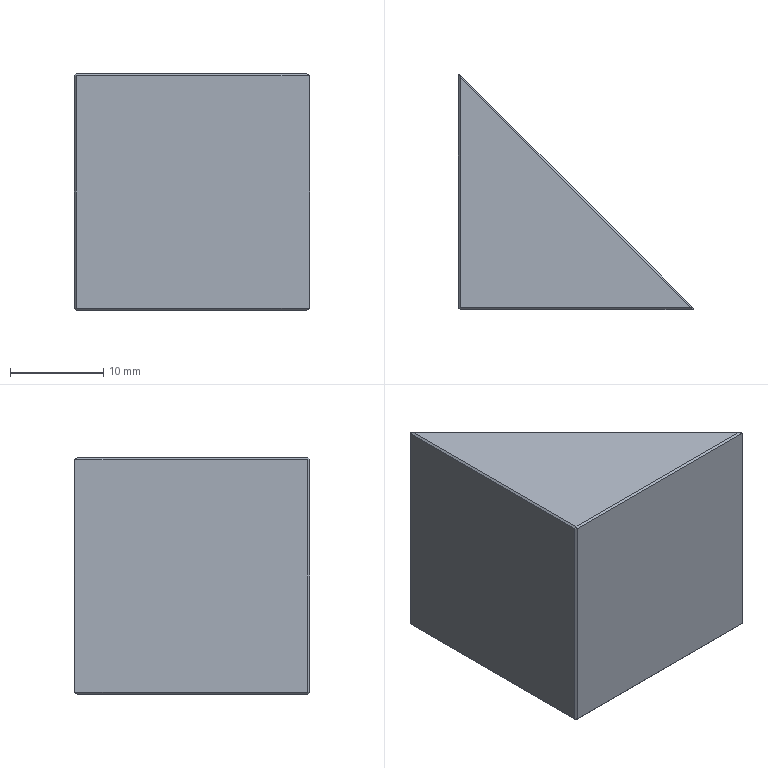Part | STEP file | PBS24-532-HP-1-0.step.STEP.STEP-259.STEP | 1 solid | 20 faces | box 25.259 x 25.259 x 25.4 mm | volume 8189 mm3 | plane 20
STEP:
#1=CARTESIAN_POINT('',(25.201,0.002851,25.203));
#2=VERTEX_POINT('',#1);
#3=CARTESIAN_POINT('',(25.257,0.1386,25.203));
#4=VERTEX_POINT('',#3);
#5=CARTESIAN_POINT('',(25.259,0.1414,25.203));
#6=DIRECTION('',(0.3827,0.9239,0.));
#7=VECTOR('',#6,1000.);
#8=LINE('',#5,#7);
#9=EDGE_CURVE('',#2,#4,#8,.T.);
#10=ORIENTED_EDGE('',*,*,#9,.F.);
#11=CARTESIAN_POINT('',(25.2,0.,25.2));
#12=VERTEX_POINT('',#11);
#13=CARTESIAN_POINT('',(25.27,0.1684,25.368));
#14=DIRECTION('',(-0.2811,-0.6786,-0.6786));
#15=VECTOR('',#14,1000.);
#16=LINE('',#13,#15);
#17=EDGE_CURVE('',#2,#12,#16,.T.);
#18=ORIENTED_EDGE('',*,*,#17,.T.);
#19=CARTESIAN_POINT('',(25.2,0.,0.2));
#20=VERTEX_POINT('',#19);
#21=CARTESIAN_POINT('',(25.2,0.,25.4));
#22=DIRECTION('',(0.,0.,1.));
#23=VECTOR('',#22,1000.);
#24=LINE('',#21,#23);
#25=EDGE_CURVE('',#20,#12,#24,.T.);
#26=ORIENTED_EDGE('',*,*,#25,.F.);
#27=CARTESIAN_POINT('',(25.201,0.002851,0.1971));
#28=VERTEX_POINT('',#27);
#29=CARTESIAN_POINT('',(20.425,-11.528,11.728));
#30=DIRECTION('',(0.2811,0.6786,-0.6786));
#31=VECTOR('',#30,1000.);
#32=LINE('',#29,#31);
#33=EDGE_CURVE('',#20,#28,#32,.T.);
#34=ORIENTED_EDGE('',*,*,#33,.T.);
#35=CARTESIAN_POINT('',(25.257,0.1386,0.1971));
#36=VERTEX_POINT('',#35);
#37=CARTESIAN_POINT('',(25.259,0.1414,0.1971));
#38=DIRECTION('',(0.3827,0.9239,0.));
#39=VECTOR('',#38,1000.);
#40=LINE('',#37,#39);
#41=EDGE_CURVE('',#28,#36,#40,.T.);
#42=ORIENTED_EDGE('',*,*,#41,.T.);
#43=CARTESIAN_POINT('',(25.259,0.1414,0.2));
#44=VERTEX_POINT('',#43);
#45=CARTESIAN_POINT('',(28.081,6.955,7.014));
#46=DIRECTION('',(-0.2811,-0.6786,-0.6786));
#47=VECTOR('',#46,1000.);
#48=LINE('',#45,#47);
#49=EDGE_CURVE('',#44,#36,#48,.T.);
#50=ORIENTED_EDGE('',*,*,#49,.F.);
#51=CARTESIAN_POINT('',(25.259,0.1414,25.2));
#52=VERTEX_POINT('',#51);
#53=CARTESIAN_POINT('',(25.259,0.1414,25.4));
#54=DIRECTION('',(0.,0.,-1.));
#55=VECTOR('',#54,1000.);
#56=LINE('',#53,#55);
#57=EDGE_CURVE('',#52,#44,#56,.T.);
#58=ORIENTED_EDGE('',*,*,#57,.F.);
#59=CARTESIAN_POINT('',(26.586,3.345,21.996));
#60=DIRECTION('',(0.2811,0.6786,-0.6786));
#61=VECTOR('',#60,1000.);
#62=LINE('',#59,#61);
#63=EDGE_CURVE('',#4,#52,#62,.T.);
#64=ORIENTED_EDGE('',*,*,#63,.F.);
#65=EDGE_LOOP('',(#10,#18,#26,#34,#42,#50,#58,#64));
#66=FACE_OUTER_BOUND('',#65,.T.);
#67=CARTESIAN_POINT('',(25.259,0.1414,25.4));
#68=DIRECTION('',(-0.9239,0.3827,0.));
#69=DIRECTION('',(0.,0.,1.));
#70=AXIS2_PLACEMENT_3D('',#67,#68,#69);
#71=PLANE('',#70);
#72=ADVANCED_FACE('',(#66),#71,.F.);
#73=CARTESIAN_POINT('',(24.919,0.1994,0.0006229));
#74=VERTEX_POINT('',#73);
#75=CARTESIAN_POINT('',(24.917,0.2,0.));
#76=VERTEX_POINT('',#75);
#77=CARTESIAN_POINT('',(-1.344,11.078,-10.878));
#78=DIRECTION('',(-0.8629,0.3574,-0.3574));
#79=VECTOR('',#78,1000.);
#80=LINE('',#77,#79);
#81=EDGE_CURVE('',#74,#76,#80,.T.);
#82=ORIENTED_EDGE('',*,*,#81,.F.);
#83=CARTESIAN_POINT('',(12.396,8.91,-8.71));
#84=DIRECTION('',(0.7129,-0.4959,0.4959));
#85=VECTOR('',#84,1000.);
#86=LINE('',#83,#85);
#87=EDGE_CURVE('',#74,#28,#86,.T.);
#88=ORIENTED_EDGE('',*,*,#87,.T.);
#89=ORIENTED_EDGE('',*,*,#33,.F.);
#90=CARTESIAN_POINT('',(0.2,0.,0.2));
#91=VERTEX_POINT('',#90);
#92=CARTESIAN_POINT('',(25.117,0.,0.2));
#93=DIRECTION('',(1.,0.,0.));
#94=VECTOR('',#93,1000.);
#95=LINE('',#92,#94);
#96=EDGE_CURVE('',#91,#20,#95,.T.);
#97=ORIENTED_EDGE('',*,*,#96,.F.);
#98=CARTESIAN_POINT('',(0.1981,0.00185,0.1981));
#99=VERTEX_POINT('',#98);
#100=CARTESIAN_POINT('',(8.6,-8.4,8.6));
#101=DIRECTION('',(0.5774,-0.5774,0.5774));
#102=VECTOR('',#101,1000.);
#103=LINE('',#100,#102);
#104=EDGE_CURVE('',#99,#91,#103,.T.);
#105=ORIENTED_EDGE('',*,*,#104,.F.);
#106=CARTESIAN_POINT('',(0.1981,0.1981,0.00185));
#107=VERTEX_POINT('',#106);
#108=CARTESIAN_POINT('',(0.1981,0.,0.2));
#109=DIRECTION('',(0.,0.7071,-0.7071));
#110=VECTOR('',#109,1000.);
#111=LINE('',#108,#110);
#112=EDGE_CURVE('',#99,#107,#111,.T.);
#113=ORIENTED_EDGE('',*,*,#112,.T.);
#114=CARTESIAN_POINT('',(0.2,0.2,0.));
#115=VERTEX_POINT('',#114);
#116=CARTESIAN_POINT('',(0.,0.,0.2));
#117=DIRECTION('',(-0.5774,-0.5774,0.5774));
#118=VECTOR('',#117,1000.);
#119=LINE('',#116,#118);
#120=EDGE_CURVE('',#115,#107,#119,.T.);
#121=ORIENTED_EDGE('',*,*,#120,.F.);
#122=CARTESIAN_POINT('',(0.2,0.2,0.));
#123=DIRECTION('',(-1.,0.,0.));
#124=VECTOR('',#123,1000.);
#125=LINE('',#122,#124);
#126=EDGE_CURVE('',#76,#115,#125,.T.);
#127=ORIENTED_EDGE('',*,*,#126,.F.);
#128=EDGE_LOOP('',(#82,#88,#89,#97,#105,#113,#121,#127));
#129=FACE_OUTER_BOUND('',#128,.T.);
#130=CARTESIAN_POINT('',(0.,0.,0.2));
#131=DIRECTION('',(0.,-0.7071,-0.7071));
#132=DIRECTION('',(0.,-0.7071,0.7071));
#133=AXIS2_PLACEMENT_3D('',#130,#131,#132);
#134=PLANE('',#133);
#135=ADVANCED_FACE('',(#129),#134,.T.);
#136=ORIENTED_EDGE('',*,*,#49,.T.);
#137=CARTESIAN_POINT('',(3.494,4.045,-12.429));
#138=DIRECTION('',(-0.8547,0.1534,-0.4959));
#139=VECTOR('',#138,1000.);
#140=LINE('',#137,#139);
#141=EDGE_CURVE('',#36,#74,#140,.T.);
#142=ORIENTED_EDGE('',*,*,#141,.T.);
#143=ORIENTED_EDGE('',*,*,#81,.T.);
#144=CARTESIAN_POINT('',(0.2,24.917,0.));
#145=VERTEX_POINT('',#144);
#146=CARTESIAN_POINT('',(25.259,-0.1414,0.));
#147=DIRECTION('',(0.7071,-0.7071,0.));
#148=VECTOR('',#147,1000.);
#149=LINE('',#146,#148);
#150=EDGE_CURVE('',#145,#76,#149,.T.);
#151=ORIENTED_EDGE('',*,*,#150,.F.);
#152=CARTESIAN_POINT('',(0.1994,24.919,0.0006229));
#153=VERTEX_POINT('',#152);
#154=CARTESIAN_POINT('',(0.,25.4,0.2));
#155=DIRECTION('',(-0.3574,0.8629,0.3574));
#156=VECTOR('',#155,1000.);
#157=LINE('',#154,#156);
#158=EDGE_CURVE('',#145,#153,#157,.T.);
#159=ORIENTED_EDGE('',*,*,#158,.T.);
#160=CARTESIAN_POINT('',(0.1386,25.257,0.1971));
#161=VERTEX_POINT('',#160);
#162=CARTESIAN_POINT('',(0.1164,25.381,0.2688));
#163=DIRECTION('',(-0.1534,0.8547,0.4959));
#164=VECTOR('',#163,1000.);
#165=LINE('',#162,#164);
#166=EDGE_CURVE('',#153,#161,#165,.T.);
#167=ORIENTED_EDGE('',*,*,#166,.T.);
#168=CARTESIAN_POINT('',(0.1414,25.259,0.2));
#169=VERTEX_POINT('',#168);
#170=CARTESIAN_POINT('',(0.1033,25.243,0.1619));
#171=DIRECTION('',(0.6786,0.2811,0.6786));
#172=VECTOR('',#171,1000.);
#173=LINE('',#170,#172);
#174=EDGE_CURVE('',#161,#169,#173,.T.);
#175=ORIENTED_EDGE('',*,*,#174,.T.);
#176=CARTESIAN_POINT('',(0.,25.4,0.2));
#177=DIRECTION('',(-0.7071,0.7071,0.));
#178=VECTOR('',#177,1000.);
#179=LINE('',#176,#178);
#180=EDGE_CURVE('',#44,#169,#179,.T.);
#181=ORIENTED_EDGE('',*,*,#180,.F.);
#182=EDGE_LOOP('',(#136,#142,#143,#151,#159,#167,#175,#181));
#183=FACE_OUTER_BOUND('',#182,.T.);
#184=CARTESIAN_POINT('',(0.,25.4,0.2));
#185=DIRECTION('',(0.5,0.5,-0.7071));
#186=DIRECTION('',(-0.8165,0.,-0.5774));
#187=AXIS2_PLACEMENT_3D('',#184,#185,#186);
#188=PLANE('',#187);
#189=ADVANCED_FACE('',(#183),#188,.T.);
#190=CARTESIAN_POINT('',(0.,25.2,0.2));
#191=VERTEX_POINT('',#190);
#192=CARTESIAN_POINT('',(0.002851,25.201,0.1971));
#193=VERTEX_POINT('',#192);
#194=CARTESIAN_POINT('',(-4.807,23.209,5.007));
#195=DIRECTION('',(0.6786,0.2811,-0.6786));
#196=VECTOR('',#195,1000.);
#197=LINE('',#194,#196);
#198=EDGE_CURVE('',#191,#193,#197,.T.);
#199=ORIENTED_EDGE('',*,*,#198,.T.);
#200=CARTESIAN_POINT('',(8.91,12.396,-8.71));
#201=DIRECTION('',(0.4959,-0.7129,-0.4959));
#202=VECTOR('',#201,1000.);
#203=LINE('',#200,#202);
#204=EDGE_CURVE('',#193,#153,#203,.T.);
#205=ORIENTED_EDGE('',*,*,#204,.T.);
#206=ORIENTED_EDGE('',*,*,#158,.F.);
#207=CARTESIAN_POINT('',(0.2,25.117,0.));
#208=DIRECTION('',(0.,1.,0.));
#209=VECTOR('',#208,1000.);
#210=LINE('',#207,#209);
#211=EDGE_CURVE('',#115,#145,#210,.T.);
#212=ORIENTED_EDGE('',*,*,#211,.F.);
#213=ORIENTED_EDGE('',*,*,#120,.T.);
#214=CARTESIAN_POINT('',(0.00185,0.1981,0.1981));
#215=VERTEX_POINT('',#214);
#216=CARTESIAN_POINT('',(0.,0.1981,0.2));
#217=DIRECTION('',(-0.7071,0.,0.7071));
#218=VECTOR('',#217,1000.);
#219=LINE('',#216,#218);
#220=EDGE_CURVE('',#107,#215,#219,.T.);
#221=ORIENTED_EDGE('',*,*,#220,.T.);
#222=CARTESIAN_POINT('',(0.,0.2,0.2));
#223=VERTEX_POINT('',#222);
#224=CARTESIAN_POINT('',(0.06667,0.1333,0.1333));
#225=DIRECTION('',(-0.5774,0.5774,0.5774));
#226=VECTOR('',#225,1000.);
#227=LINE('',#224,#226);
#228=EDGE_CURVE('',#215,#223,#227,.T.);
#229=ORIENTED_EDGE('',*,*,#228,.T.);
#230=CARTESIAN_POINT('',(0.,0.,0.2));
#231=DIRECTION('',(0.,-1.,0.));
#232=VECTOR('',#231,1000.);
#233=LINE('',#230,#232);
#234=EDGE_CURVE('',#191,#223,#233,.T.);
#235=ORIENTED_EDGE('',*,*,#234,.F.);
#236=EDGE_LOOP('',(#199,#205,#206,#212,#213,#221,#229,#235));
#237=FACE_OUTER_BOUND('',#236,.T.);
#238=CARTESIAN_POINT('',(0.,0.,0.2));
#239=DIRECTION('',(-0.7071,0.,-0.7071));
#240=DIRECTION('',(-0.7071,0.,0.7071));
#241=AXIS2_PLACEMENT_3D('',#238,#239,#240);
#242=PLANE('',#241);
#243=ADVANCED_FACE('',(#237),#242,.T.);
#244=ORIENTED_EDGE('',*,*,#174,.F.);
#245=CARTESIAN_POINT('',(0.,25.2,0.1971));
#246=DIRECTION('',(-0.9239,-0.3827,0.));
#247=VECTOR('',#246,1000.);
#248=LINE('',#245,#247);
#249=EDGE_CURVE('',#161,#193,#248,.T.);
#250=ORIENTED_EDGE('',*,*,#249,.T.);
#251=ORIENTED_EDGE('',*,*,#198,.F.);
#252=CARTESIAN_POINT('',(0.,25.2,25.2));
#253=VERTEX_POINT('',#252);
#254=CARTESIAN_POINT('',(0.,25.2,25.4));
#255=DIRECTION('',(0.,0.,-1.));
#256=VECTOR('',#255,1000.);
#257=LINE('',#254,#256);
#258=EDGE_CURVE('',#253,#191,#257,.T.);
#259=ORIENTED_EDGE('',*,*,#258,.F.);
#260=CARTESIAN_POINT('',(0.002851,25.201,25.203));
#261=VERTEX_POINT('',#260);
#262=CARTESIAN_POINT('',(-4.623,23.285,20.577));
#263=DIRECTION('',(-0.6786,-0.2811,-0.6786));
#264=VECTOR('',#263,1000.);
#265=LINE('',#262,#264);
#266=EDGE_CURVE('',#261,#253,#265,.T.);
#267=ORIENTED_EDGE('',*,*,#266,.F.);
#268=CARTESIAN_POINT('',(0.1386,25.257,25.203));
#269=VERTEX_POINT('',#268);
#270=CARTESIAN_POINT('',(0.,25.2,25.203));
#271=DIRECTION('',(0.9239,0.3827,0.));
#272=VECTOR('',#271,1000.);
#273=LINE('',#270,#272);
#274=EDGE_CURVE('',#261,#269,#273,.T.);
#275=ORIENTED_EDGE('',*,*,#274,.T.);
#276=CARTESIAN_POINT('',(0.1414,25.259,25.2));
#277=VERTEX_POINT('',#276);
#278=CARTESIAN_POINT('',(3.345,26.586,21.996));
#279=DIRECTION('',(-0.6786,-0.2811,0.6786));
#280=VECTOR('',#279,1000.);
#281=LINE('',#278,#280);
#282=EDGE_CURVE('',#277,#269,#281,.T.);
#283=ORIENTED_EDGE('',*,*,#282,.F.);
#284=CARTESIAN_POINT('',(0.1414,25.259,25.4));
#285=DIRECTION('',(0.,0.,1.));
#286=VECTOR('',#285,1000.);
#287=LINE('',#284,#286);
#288=EDGE_CURVE('',#169,#277,#287,.T.);
#289=ORIENTED_EDGE('',*,*,#288,.F.);
#290=EDGE_LOOP('',(#244,#250,#251,#259,#267,#275,#283,#289));
#291=FACE_OUTER_BOUND('',#290,.T.);
#292=CARTESIAN_POINT('',(0.,25.2,25.4));
#293=DIRECTION('',(0.3827,-0.9239,0.));
#294=DIRECTION('',(0.,0.,-1.));
#295=AXIS2_PLACEMENT_3D('',#292,#293,#294);
#296=PLANE('',#295);
#297=ADVANCED_FACE('',(#291),#296,.F.);
#298=CARTESIAN_POINT('',(24.919,0.1994,25.399));
#299=VERTEX_POINT('',#298);
#300=CARTESIAN_POINT('',(14.268,2.111,31.579));
#301=DIRECTION('',(-0.8547,0.1534,0.4959));
#302=VECTOR('',#301,1000.);
#303=LINE('',#300,#302);
#304=EDGE_CURVE('',#4,#299,#303,.T.);
#305=ORIENTED_EDGE('',*,*,#304,.F.);
#306=ORIENTED_EDGE('',*,*,#63,.T.);
#307=CARTESIAN_POINT('',(0.,25.4,25.2));
#308=DIRECTION('',(0.7071,-0.7071,0.));
#309=VECTOR('',#308,1000.);
#310=LINE('',#307,#309);
#311=EDGE_CURVE('',#277,#52,#310,.T.);
#312=ORIENTED_EDGE('',*,*,#311,.F.);
#313=ORIENTED_EDGE('',*,*,#282,.T.);
#314=CARTESIAN_POINT('',(0.1994,24.919,25.399));
#315=VERTEX_POINT('',#314);
#316=CARTESIAN_POINT('',(2.111,14.268,31.579));
#317=DIRECTION('',(0.1534,-0.8547,0.4959));
#318=VECTOR('',#317,1000.);
#319=LINE('',#316,#318);
#320=EDGE_CURVE('',#269,#315,#319,.T.);
#321=ORIENTED_EDGE('',*,*,#320,.T.);
#322=CARTESIAN_POINT('',(0.2,24.917,25.4));
#323=VERTEX_POINT('',#322);
#324=CARTESIAN_POINT('',(5.59,11.905,30.79));
#325=DIRECTION('',(0.3574,-0.8629,0.3574));
#326=VECTOR('',#325,1000.);
#327=LINE('',#324,#326);
#328=EDGE_CURVE('',#315,#323,#327,.T.);
#329=ORIENTED_EDGE('',*,*,#328,.T.);
#330=CARTESIAN_POINT('',(24.917,0.2,25.4));
#331=VERTEX_POINT('',#330);
#332=CARTESIAN_POINT('',(12.559,12.559,25.4));
#333=DIRECTION('',(-0.7071,0.7071,0.));
#334=VECTOR('',#333,1000.);
#335=LINE('',#332,#334);
#336=EDGE_CURVE('',#331,#323,#335,.T.);
#337=ORIENTED_EDGE('',*,*,#336,.F.);
#338=CARTESIAN_POINT('',(11.905,5.59,30.79));
#339=DIRECTION('',(0.8629,-0.3574,-0.3574));
#340=VECTOR('',#339,1000.);
#341=LINE('',#338,#340);
#342=EDGE_CURVE('',#331,#299,#341,.T.);
#343=ORIENTED_EDGE('',*,*,#342,.T.);
#344=EDGE_LOOP('',(#305,#306,#312,#313,#321,#329,#337,#343));
#345=FACE_OUTER_BOUND('',#344,.T.);
#346=CARTESIAN_POINT('',(12.559,12.559,25.4));
#347=DIRECTION('',(-0.5,-0.5,-0.7071));
#348=DIRECTION('',(0.,-0.8165,0.5774));
#349=AXIS2_PLACEMENT_3D('',#346,#347,#348);
#350=PLANE('',#349);
#351=ADVANCED_FACE('',(#345),#350,.F.);
#352=ORIENTED_EDGE('',*,*,#328,.F.);
#353=CARTESIAN_POINT('',(9.009,12.255,34.209));
#354=DIRECTION('',(-0.4959,0.7129,-0.4959));
#355=VECTOR('',#354,1000.);
#356=LINE('',#353,#355);
#357=EDGE_CURVE('',#315,#261,#356,.T.);
#358=ORIENTED_EDGE('',*,*,#357,.T.);
#359=ORIENTED_EDGE('',*,*,#266,.T.);
#360=CARTESIAN_POINT('',(0.,0.2,25.2));
#361=VERTEX_POINT('',#360);
#362=CARTESIAN_POINT('',(0.,0.,25.2));
#363=DIRECTION('',(0.,1.,0.));
#364=VECTOR('',#363,1000.);
#365=LINE('',#362,#364);
#366=EDGE_CURVE('',#361,#253,#365,.T.);
#367=ORIENTED_EDGE('',*,*,#366,.F.);
#368=CARTESIAN_POINT('',(0.00185,0.1981,25.202));
#369=VERTEX_POINT('',#368);
#370=CARTESIAN_POINT('',(0.2,0.,25.4));
#371=DIRECTION('',(0.5774,-0.5774,0.5774));
#372=VECTOR('',#371,1000.);
#373=LINE('',#370,#372);
#374=EDGE_CURVE('',#361,#369,#373,.T.);
#375=ORIENTED_EDGE('',*,*,#374,.T.);
#376=CARTESIAN_POINT('',(0.1981,0.1981,25.398));
#377=VERTEX_POINT('',#376);
#378=CARTESIAN_POINT('',(0.2,0.1981,25.4));
#379=DIRECTION('',(0.7071,0.,0.7071));
#380=VECTOR('',#379,1000.);
#381=LINE('',#378,#380);
#382=EDGE_CURVE('',#369,#377,#381,.T.);
#383=ORIENTED_EDGE('',*,*,#382,.T.);
#384=CARTESIAN_POINT('',(0.2,0.2,25.4));
#385=VERTEX_POINT('',#384);
#386=CARTESIAN_POINT('',(0.1333,0.1333,25.333));
#387=DIRECTION('',(0.5774,0.5774,0.5774));
#388=VECTOR('',#387,1000.);
#389=LINE('',#386,#388);
#390=EDGE_CURVE('',#377,#385,#389,.T.);
#391=ORIENTED_EDGE('',*,*,#390,.T.);
#392=CARTESIAN_POINT('',(0.2,0.,25.4));
#393=DIRECTION('',(0.,-1.,0.));
#394=VECTOR('',#393,1000.);
#395=LINE('',#392,#394);
#396=EDGE_CURVE('',#323,#385,#395,.T.);
#397=ORIENTED_EDGE('',*,*,#396,.F.);
#398=EDGE_LOOP('',(#352,#358,#359,#367,#375,#383,#391,#397));
#399=FACE_OUTER_BOUND('',#398,.T.);
#400=CARTESIAN_POINT('',(0.2,0.,25.4));
#401=DIRECTION('',(0.7071,0.,-0.7071));
#402=DIRECTION('',(0.,-1.,0.));
#403=AXIS2_PLACEMENT_3D('',#400,#401,#402);
#404=PLANE('',#403);
#405=ADVANCED_FACE('',(#399),#404,.F.);
#406=ORIENTED_EDGE('',*,*,#228,.F.);
#407=CARTESIAN_POINT('',(0.2,0.,0.1981));
#408=DIRECTION('',(0.7071,-0.7071,0.));
#409=VECTOR('',#408,1000.);
#410=LINE('',#407,#409);
#411=EDGE_CURVE('',#215,#99,#410,.T.);
#412=ORIENTED_EDGE('',*,*,#411,.T.);
#413=ORIENTED_EDGE('',*,*,#104,.T.);
#414=CARTESIAN_POINT('',(0.2,0.,25.2));
#415=VERTEX_POINT('',#414);
#416=CARTESIAN_POINT('',(0.2,0.,25.4));
#417=DIRECTION('',(0.,0.,-1.));
#418=VECTOR('',#417,1000.);
#419=LINE('',#416,#418);
#420=EDGE_CURVE('',#415,#91,#419,.T.);
#421=ORIENTED_EDGE('',*,*,#420,.F.);
#422=CARTESIAN_POINT('',(0.1981,0.00185,25.202));
#423=VERTEX_POINT('',#422);
#424=CARTESIAN_POINT('',(0.1333,0.06667,25.267));
#425=DIRECTION('',(-0.5774,0.5774,0.5774));
#426=VECTOR('',#425,1000.);
#427=LINE('',#424,#426);
#428=EDGE_CURVE('',#415,#423,#427,.T.);
#429=ORIENTED_EDGE('',*,*,#428,.T.);
#430=CARTESIAN_POINT('',(0.2,0.,25.202));
#431=DIRECTION('',(-0.7071,0.7071,0.));
#432=VECTOR('',#431,1000.);
#433=LINE('',#430,#432);
#434=EDGE_CURVE('',#423,#369,#433,.T.);
#435=ORIENTED_EDGE('',*,*,#434,.T.);
#436=ORIENTED_EDGE('',*,*,#374,.F.);
#437=CARTESIAN_POINT('',(0.,0.2,25.4));
#438=DIRECTION('',(0.,0.,1.));
#439=VECTOR('',#438,1000.);
#440=LINE('',#437,#439);
#441=EDGE_CURVE('',#223,#361,#440,.T.);
#442=ORIENTED_EDGE('',*,*,#441,.F.);
#443=EDGE_LOOP('',(#406,#412,#413,#421,#429,#435,#436,#442));
#444=FACE_OUTER_BOUND('',#443,.T.);
#445=CARTESIAN_POINT('',(0.2,0.,25.4));
#446=DIRECTION('',(0.7071,0.7071,0.));
#447=DIRECTION('',(0.,0.,-1.));
#448=AXIS2_PLACEMENT_3D('',#445,#446,#447);
#449=PLANE('',#448);
#450=ADVANCED_FACE('',(#444),#449,.F.);
#451=CARTESIAN_POINT('',(12.255,9.009,34.209));
#452=DIRECTION('',(0.7129,-0.4959,-0.4959));
#453=VECTOR('',#452,1000.);
#454=LINE('',#451,#453);
#455=EDGE_CURVE('',#299,#2,#454,.T.);
#456=ORIENTED_EDGE('',*,*,#455,.F.);
#457=ORIENTED_EDGE('',*,*,#342,.F.);
#458=CARTESIAN_POINT('',(0.,0.2,25.4));
#459=DIRECTION('',(1.,0.,0.));
#460=VECTOR('',#459,1000.);
#461=LINE('',#458,#460);
#462=EDGE_CURVE('',#385,#331,#461,.T.);
#463=ORIENTED_EDGE('',*,*,#462,.F.);
#464=ORIENTED_EDGE('',*,*,#390,.F.);
#465=CARTESIAN_POINT('',(0.1981,0.2,25.4));
#466=DIRECTION('',(0.,-0.7071,-0.7071));
#467=VECTOR('',#466,1000.);
#468=LINE('',#465,#467);
#469=EDGE_CURVE('',#377,#423,#468,.T.);
#470=ORIENTED_EDGE('',*,*,#469,.T.);
#471=ORIENTED_EDGE('',*,*,#428,.F.);
#472=CARTESIAN_POINT('',(0.,0.,25.2));
#473=DIRECTION('',(-1.,0.,0.));
#474=VECTOR('',#473,1000.);
#475=LINE('',#472,#474);
#476=EDGE_CURVE('',#12,#415,#475,.T.);
#477=ORIENTED_EDGE('',*,*,#476,.F.);
#478=ORIENTED_EDGE('',*,*,#17,.F.);
#479=EDGE_LOOP('',(#456,#457,#463,#464,#470,#471,#477,#478));
#480=FACE_OUTER_BOUND('',#479,.T.);
#481=CARTESIAN_POINT('',(0.,0.2,25.4));
#482=DIRECTION('',(0.,0.7071,-0.7071));
#483=DIRECTION('',(-1.,0.,0.));
#484=AXIS2_PLACEMENT_3D('',#481,#482,#483);
#485=PLANE('',#484);
#486=ADVANCED_FACE('',(#480),#485,.F.);
#487=ORIENTED_EDGE('',*,*,#366,.T.);
#488=ORIENTED_EDGE('',*,*,#258,.T.);
#489=ORIENTED_EDGE('',*,*,#234,.T.);
#490=ORIENTED_EDGE('',*,*,#441,.T.);
#491=EDGE_LOOP('',(#487,#488,#489,#490));
#492=FACE_OUTER_BOUND('',#491,.T.);
#493=CARTESIAN_POINT('',(0.,0.,25.4));
#494=DIRECTION('',(1.,0.,0.));
#495=DIRECTION('',(0.,1.,0.));
#496=AXIS2_PLACEMENT_3D('',#493,#494,#495);
#497=PLANE('',#496);
#498=ADVANCED_FACE('',(#492),#497,.F.);
#499=ORIENTED_EDGE('',*,*,#25,.T.);
#500=ORIENTED_EDGE('',*,*,#476,.T.);
#501=ORIENTED_EDGE('',*,*,#420,.T.);
#502=ORIENTED_EDGE('',*,*,#96,.T.);
#503=EDGE_LOOP('',(#499,#500,#501,#502));
#504=FACE_OUTER_BOUND('',#503,.T.);
#505=CARTESIAN_POINT('',(0.,0.,25.4));
#506=DIRECTION('',(0.,1.,0.));
#507=DIRECTION('',(1.,0.,0.));
#508=AXIS2_PLACEMENT_3D('',#505,#506,#507);
#509=PLANE('',#508);
#510=ADVANCED_FACE('',(#504),#509,.F.);
#511=ORIENTED_EDGE('',*,*,#180,.T.);
#512=ORIENTED_EDGE('',*,*,#288,.T.);
#513=ORIENTED_EDGE('',*,*,#311,.T.);
#514=ORIENTED_EDGE('',*,*,#57,.T.);
#515=EDGE_LOOP('',(#511,#512,#513,#514));
#516=FACE_OUTER_BOUND('',#515,.T.);
#517=CARTESIAN_POINT('',(0.,25.4,25.4));
#518=DIRECTION('',(-0.7071,-0.7071,0.));
#519=DIRECTION('',(-0.7071,0.7071,0.));
#520=AXIS2_PLACEMENT_3D('',#517,#518,#519);
#521=PLANE('',#520);
#522=ADVANCED_FACE('',(#516),#521,.F.);
#523=ORIENTED_EDGE('',*,*,#396,.T.);
#524=ORIENTED_EDGE('',*,*,#462,.T.);
#525=ORIENTED_EDGE('',*,*,#336,.T.);
#526=EDGE_LOOP('',(#523,#524,#525));
#527=FACE_OUTER_BOUND('',#526,.T.);
#528=CARTESIAN_POINT('',(0.,0.,25.4));
#529=DIRECTION('',(0.,0.,-1.));
#530=DIRECTION('',(0.,-1.,0.));
#531=AXIS2_PLACEMENT_3D('',#528,#529,#530);
#532=PLANE('',#531);
#533=ADVANCED_FACE('',(#527),#532,.F.);
#534=ORIENTED_EDGE('',*,*,#150,.T.);
#535=ORIENTED_EDGE('',*,*,#126,.T.);
#536=ORIENTED_EDGE('',*,*,#211,.T.);
#537=EDGE_LOOP('',(#534,#535,#536));
#538=FACE_OUTER_BOUND('',#537,.T.);
#539=CARTESIAN_POINT('',(0.,0.,0.));
#540=DIRECTION('',(0.,0.,-1.));
#541=DIRECTION('',(0.,-1.,0.));
#542=AXIS2_PLACEMENT_3D('',#539,#540,#541);
#543=PLANE('',#542);
#544=ADVANCED_FACE('',(#538),#543,.T.);
#545=ORIENTED_EDGE('',*,*,#382,.F.);
#546=ORIENTED_EDGE('',*,*,#434,.F.);
#547=ORIENTED_EDGE('',*,*,#469,.F.);
#548=EDGE_LOOP('',(#545,#546,#547));
#549=FACE_OUTER_BOUND('',#548,.T.);
#550=CARTESIAN_POINT('',(-8.334,-8.334,8.334));
#551=DIRECTION('',(-0.5774,-0.5774,0.5774));
#552=DIRECTION('',(-0.7071,0.7071,0.));
#553=AXIS2_PLACEMENT_3D('',#550,#551,#552);
#554=PLANE('',#553);
#555=ADVANCED_FACE('',(#549),#554,.T.);
#556=ORIENTED_EDGE('',*,*,#411,.F.);
#557=ORIENTED_EDGE('',*,*,#220,.F.);
#558=ORIENTED_EDGE('',*,*,#112,.F.);
#559=EDGE_LOOP('',(#556,#557,#558));
#560=FACE_OUTER_BOUND('',#559,.T.);
#561=CARTESIAN_POINT('',(0.1327,0.1327,0.1327));
#562=DIRECTION('',(-0.5774,-0.5774,-0.5774));
#563=DIRECTION('',(0.,-0.7071,0.7071));
#564=AXIS2_PLACEMENT_3D('',#561,#562,#563);
#565=PLANE('',#564);
#566=ADVANCED_FACE('',(#560),#565,.T.);
#567=ORIENTED_EDGE('',*,*,#357,.F.);
#568=ORIENTED_EDGE('',*,*,#320,.F.);
#569=ORIENTED_EDGE('',*,*,#274,.F.);
#570=EDGE_LOOP('',(#567,#568,#569));
#571=FACE_OUTER_BOUND('',#570,.T.);
#572=CARTESIAN_POINT('',(-6.471,15.622,28.928));
#573=DIRECTION('',(-0.1931,0.4662,0.8633));
#574=DIRECTION('',(0.9239,0.3827,0.));
#575=AXIS2_PLACEMENT_3D('',#572,#573,#574);
#576=PLANE('',#575);
#577=ADVANCED_FACE('',(#571),#576,.T.);
#578=ORIENTED_EDGE('',*,*,#249,.F.);
#579=ORIENTED_EDGE('',*,*,#166,.F.);
#580=ORIENTED_EDGE('',*,*,#204,.F.);
#581=EDGE_LOOP('',(#578,#579,#580));
#582=FACE_OUTER_BOUND('',#581,.T.);
#583=CARTESIAN_POINT('',(-2.236,5.398,-9.996));
#584=DIRECTION('',(-0.1931,0.4662,-0.8633));
#585=DIRECTION('',(-0.9759,0.,0.2183));
#586=AXIS2_PLACEMENT_3D('',#583,#584,#585);
#587=PLANE('',#586);
#588=ADVANCED_FACE('',(#582),#587,.T.);
#589=ORIENTED_EDGE('',*,*,#141,.F.);
#590=ORIENTED_EDGE('',*,*,#41,.F.);
#591=ORIENTED_EDGE('',*,*,#87,.F.);
#592=EDGE_LOOP('',(#589,#590,#591));
#593=FACE_OUTER_BOUND('',#592,.T.);
#594=CARTESIAN_POINT('',(5.398,-2.236,-9.996));
#595=DIRECTION('',(0.4662,-0.1931,-0.8633));
#596=DIRECTION('',(0.,-0.9759,0.2183));
#597=AXIS2_PLACEMENT_3D('',#594,#595,#596);
#598=PLANE('',#597);
#599=ADVANCED_FACE('',(#593),#598,.T.);
#600=ORIENTED_EDGE('',*,*,#455,.T.);
#601=ORIENTED_EDGE('',*,*,#9,.T.);
#602=ORIENTED_EDGE('',*,*,#304,.T.);
#603=EDGE_LOOP('',(#600,#601,#602));
#604=FACE_OUTER_BOUND('',#603,.T.);
#605=CARTESIAN_POINT('',(15.622,-6.471,28.928));
#606=DIRECTION('',(-0.4662,0.1931,-0.8633));
#607=DIRECTION('',(-0.8799,0.,0.4752));
#608=AXIS2_PLACEMENT_3D('',#605,#606,#607);
#609=PLANE('',#608);
#610=ADVANCED_FACE('',(#604),#609,.F.);
#611=CLOSED_SHELL('',(#72,#135,#189,#243,#297,#351,#405,#450,#486,#498,#510,#522,#533,#544,#555,#566,#577,#588,#599,#610));
#612=MANIFOLD_SOLID_BREP('',#611);
#613=CARTESIAN_POINT('',(0.,0.,0.));
#614=DIRECTION('',(0.,0.,1.));
#615=DIRECTION('',(1.,0.,0.));
#616=AXIS2_PLACEMENT_3D('',#613,#614,#615);
#617=(LENGTH_UNIT()NAMED_UNIT(*)SI_UNIT(.MILLI.,.METRE.));
#618=UNCERTAINTY_MEASURE_WITH_UNIT(LENGTH_MEASURE(0.00001),#617,'','');
#619=(NAMED_UNIT(*)PLANE_ANGLE_UNIT()SI_UNIT($,.RADIAN.));
#620=(NAMED_UNIT(*)SI_UNIT($,.STERADIAN.)SOLID_ANGLE_UNIT());
#621=(GEOMETRIC_REPRESENTATION_CONTEXT(3)GLOBAL_UNCERTAINTY_ASSIGNED_CONTEXT((#618))GLOBAL_UNIT_ASSIGNED_CONTEXT((#617,#619,#620))REPRESENTATION_CONTEXT('',''));
#622=ADVANCED_BREP_SHAPE_REPRESENTATION('',(#612,#616),#621);